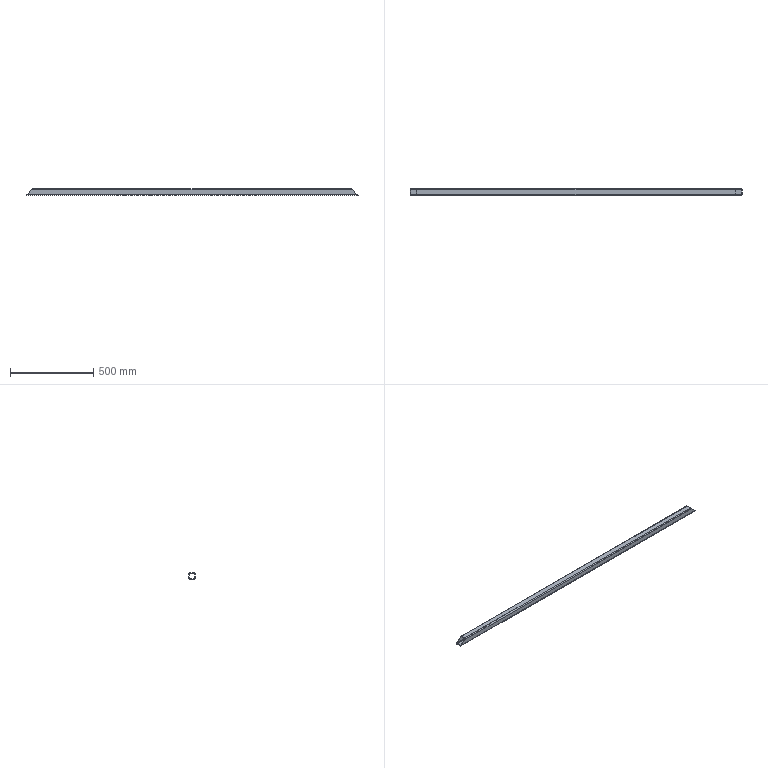Part | SolidWorks | features SavedExtBody 1 | 1 solid | 18 faces | box 2000 x 40 x 40 mm | volume 871553 mm3 | plane 10 | cylinder 8 | commonest cylinder face diameters 6.4 x4 12.8 x4
STEP:
#1=CARTESIAN_POINT('',(-1973.6,440.,-443.6));
#2=VERTEX_POINT('',#1);
#3=CARTESIAN_POINT('',(-1980.,433.6,-450.));
#4=VERTEX_POINT('',#3);
#5=CARTESIAN_POINT('',(-1973.6,440.,-443.6));
#6=CARTESIAN_POINT('',(-1977.349,440.,-447.349));
#7=CARTESIAN_POINT('',(-1980.,437.349,-450.));
#8=CARTESIAN_POINT('',(-1980.,433.6,-450.));
#9=(BOUNDED_CURVE()B_SPLINE_CURVE(3,(#5,#6,#7,#8),.UNSPECIFIED.,.F.,.F.)B_SPLINE_CURVE_WITH_KNOTS((4,4),(4.712,6.283),.UNSPECIFIED.)CURVE()GEOMETRIC_REPRESENTATION_ITEM()RATIONAL_B_SPLINE_CURVE((1.,0.8047,0.8047,1.))REPRESENTATION_ITEM(''));
#10=EDGE_CURVE('',#2,#4,#9,.T.);
#11=ORIENTED_EDGE('',*,*,#10,.F.);
#12=CARTESIAN_POINT('',(13.6,440.,-443.6));
#13=VERTEX_POINT('',#12);
#14=CARTESIAN_POINT('',(0.,440.,-443.6));
#15=DIRECTION('',(-1.,0.,0.));
#16=VECTOR('',#15,1000.);
#17=LINE('',#14,#16);
#18=EDGE_CURVE('',#13,#2,#17,.T.);
#19=ORIENTED_EDGE('',*,*,#18,.F.);
#20=CARTESIAN_POINT('',(20.,433.6,-450.));
#21=VERTEX_POINT('',#20);
#22=CARTESIAN_POINT('',(20.,433.6,-450.));
#23=CARTESIAN_POINT('',(20.,437.349,-450.));
#24=CARTESIAN_POINT('',(17.349,440.,-447.349));
#25=CARTESIAN_POINT('',(13.6,440.,-443.6));
#26=(BOUNDED_CURVE()B_SPLINE_CURVE(3,(#22,#23,#24,#25),.UNSPECIFIED.,.F.,.F.)B_SPLINE_CURVE_WITH_KNOTS((4,4),(3.142,4.712),.UNSPECIFIED.)CURVE()GEOMETRIC_REPRESENTATION_ITEM()RATIONAL_B_SPLINE_CURVE((1.,0.8047,0.8047,1.))REPRESENTATION_ITEM(''));
#27=EDGE_CURVE('',#21,#13,#26,.T.);
#28=ORIENTED_EDGE('',*,*,#27,.F.);
#29=CARTESIAN_POINT('',(0.,433.6,-450.));
#30=DIRECTION('',(-1.,0.,0.));
#31=VECTOR('',#30,1000.);
#32=LINE('',#29,#31);
#33=EDGE_CURVE('',#21,#4,#32,.T.);
#34=ORIENTED_EDGE('',*,*,#33,.T.);
#35=EDGE_LOOP('',(#11,#19,#28,#34));
#36=FACE_OUTER_BOUND('',#35,.T.);
#37=CARTESIAN_POINT('',(0.,433.6,-443.6));
#38=DIRECTION('',(-1.,0.,0.));
#39=DIRECTION('',(0.,-1.,0.));
#40=AXIS2_PLACEMENT_3D('',#37,#38,#39);
#41=CYLINDRICAL_SURFACE('',#40,6.4);
#42=ADVANCED_FACE('',(#36),#41,.T.);
#43=CARTESIAN_POINT('',(-1946.4,440.,-416.4));
#44=VERTEX_POINT('',#43);
#45=CARTESIAN_POINT('',(-986.8,440.,543.2));
#46=DIRECTION('',(-0.7071,0.,-0.7071));
#47=VECTOR('',#46,1000.);
#48=LINE('',#45,#47);
#49=EDGE_CURVE('',#44,#2,#48,.T.);
#50=ORIENTED_EDGE('',*,*,#49,.F.);
#51=CARTESIAN_POINT('',(-13.6,440.,-416.4));
#52=VERTEX_POINT('',#51);
#53=CARTESIAN_POINT('',(0.,440.,-416.4));
#54=DIRECTION('',(-1.,0.,0.));
#55=VECTOR('',#54,1000.);
#56=LINE('',#53,#55);
#57=EDGE_CURVE('',#52,#44,#56,.T.);
#58=ORIENTED_EDGE('',*,*,#57,.F.);
#59=CARTESIAN_POINT('',(6.8,440.,-436.8));
#60=DIRECTION('',(-0.7071,0.,0.7071));
#61=VECTOR('',#60,1000.);
#62=LINE('',#59,#61);
#63=EDGE_CURVE('',#13,#52,#62,.T.);
#64=ORIENTED_EDGE('',*,*,#63,.F.);
#65=ORIENTED_EDGE('',*,*,#18,.T.);
#66=EDGE_LOOP('',(#50,#58,#64,#65));
#67=FACE_OUTER_BOUND('',#66,.T.);
#68=CARTESIAN_POINT('',(0.,440.,-443.6));
#69=DIRECTION('',(0.,-1.,0.));
#70=DIRECTION('',(1.,0.,0.));
#71=AXIS2_PLACEMENT_3D('',#68,#69,#70);
#72=PLANE('',#71);
#73=ADVANCED_FACE('',(#67),#72,.F.);
#74=CARTESIAN_POINT('',(-1940.,433.6,-410.));
#75=VERTEX_POINT('',#74);
#76=CARTESIAN_POINT('',(-1940.,433.6,-410.));
#77=CARTESIAN_POINT('',(-1940.,437.349,-410.));
#78=CARTESIAN_POINT('',(-1942.651,440.,-412.651));
#79=CARTESIAN_POINT('',(-1946.4,440.,-416.4));
#80=(BOUNDED_CURVE()B_SPLINE_CURVE(3,(#76,#77,#78,#79),.UNSPECIFIED.,.F.,.F.)B_SPLINE_CURVE_WITH_KNOTS((4,4),(3.142,4.712),.UNSPECIFIED.)CURVE()GEOMETRIC_REPRESENTATION_ITEM()RATIONAL_B_SPLINE_CURVE((1.,0.8047,0.8047,1.))REPRESENTATION_ITEM(''));
#81=EDGE_CURVE('',#75,#44,#80,.T.);
#82=ORIENTED_EDGE('',*,*,#81,.F.);
#83=CARTESIAN_POINT('',(-20.,433.6,-410.));
#84=VERTEX_POINT('',#83);
#85=CARTESIAN_POINT('',(0.,433.6,-410.));
#86=DIRECTION('',(-1.,0.,0.));
#87=VECTOR('',#86,1000.);
#88=LINE('',#85,#87);
#89=EDGE_CURVE('',#84,#75,#88,.T.);
#90=ORIENTED_EDGE('',*,*,#89,.F.);
#91=CARTESIAN_POINT('',(-13.6,440.,-416.4));
#92=CARTESIAN_POINT('',(-17.349,440.,-412.651));
#93=CARTESIAN_POINT('',(-20.,437.349,-410.));
#94=CARTESIAN_POINT('',(-20.,433.6,-410.));
#95=(BOUNDED_CURVE()B_SPLINE_CURVE(3,(#91,#92,#93,#94),.UNSPECIFIED.,.F.,.F.)B_SPLINE_CURVE_WITH_KNOTS((4,4),(4.712,6.283),.UNSPECIFIED.)CURVE()GEOMETRIC_REPRESENTATION_ITEM()RATIONAL_B_SPLINE_CURVE((1.,0.8047,0.8047,1.))REPRESENTATION_ITEM(''));
#96=EDGE_CURVE('',#52,#84,#95,.T.);
#97=ORIENTED_EDGE('',*,*,#96,.F.);
#98=ORIENTED_EDGE('',*,*,#57,.T.);
#99=EDGE_LOOP('',(#82,#90,#97,#98));
#100=FACE_OUTER_BOUND('',#99,.T.);
#101=CARTESIAN_POINT('',(0.,433.6,-416.4));
#102=DIRECTION('',(-1.,0.,0.));
#103=DIRECTION('',(0.,-1.,0.));
#104=AXIS2_PLACEMENT_3D('',#101,#102,#103);
#105=CYLINDRICAL_SURFACE('',#104,6.4);
#106=ADVANCED_FACE('',(#100),#105,.T.);
#107=CARTESIAN_POINT('',(-1940.,406.4,-410.));
#108=VERTEX_POINT('',#107);
#109=CARTESIAN_POINT('',(-1940.,406.4,-410.));
#110=DIRECTION('',(0.,1.,0.));
#111=VECTOR('',#110,1000.);
#112=LINE('',#109,#111);
#113=EDGE_CURVE('',#108,#75,#112,.T.);
#114=ORIENTED_EDGE('',*,*,#113,.F.);
#115=CARTESIAN_POINT('',(-20.,406.4,-410.));
#116=VERTEX_POINT('',#115);
#117=CARTESIAN_POINT('',(0.,406.4,-410.));
#118=DIRECTION('',(-1.,0.,0.));
#119=VECTOR('',#118,1000.);
#120=LINE('',#117,#119);
#121=EDGE_CURVE('',#116,#108,#120,.T.);
#122=ORIENTED_EDGE('',*,*,#121,.F.);
#123=CARTESIAN_POINT('',(-20.,406.4,-410.));
#124=DIRECTION('',(0.,-1.,0.));
#125=VECTOR('',#124,1000.);
#126=LINE('',#123,#125);
#127=EDGE_CURVE('',#84,#116,#126,.T.);
#128=ORIENTED_EDGE('',*,*,#127,.F.);
#129=ORIENTED_EDGE('',*,*,#89,.T.);
#130=EDGE_LOOP('',(#114,#122,#128,#129));
#131=FACE_OUTER_BOUND('',#130,.T.);
#132=CARTESIAN_POINT('',(0.,406.4,-410.));
#133=DIRECTION('',(0.,0.,-1.));
#134=DIRECTION('',(0.,1.,0.));
#135=AXIS2_PLACEMENT_3D('',#132,#133,#134);
#136=PLANE('',#135);
#137=ADVANCED_FACE('',(#131),#136,.F.);
#138=CARTESIAN_POINT('',(-1946.4,400.,-416.4));
#139=VERTEX_POINT('',#138);
#140=CARTESIAN_POINT('',(-1946.4,400.,-416.4));
#141=CARTESIAN_POINT('',(-1942.651,400.,-412.651));
#142=CARTESIAN_POINT('',(-1940.,402.651,-410.));
#143=CARTESIAN_POINT('',(-1940.,406.4,-410.));
#144=(BOUNDED_CURVE()B_SPLINE_CURVE(3,(#140,#141,#142,#143),.UNSPECIFIED.,.F.,.F.)B_SPLINE_CURVE_WITH_KNOTS((4,4),(1.571,3.142),.UNSPECIFIED.)CURVE()GEOMETRIC_REPRESENTATION_ITEM()RATIONAL_B_SPLINE_CURVE((1.,0.8047,0.8047,1.))REPRESENTATION_ITEM(''));
#145=EDGE_CURVE('',#139,#108,#144,.T.);
#146=ORIENTED_EDGE('',*,*,#145,.F.);
#147=CARTESIAN_POINT('',(-13.6,400.,-416.4));
#148=VERTEX_POINT('',#147);
#149=CARTESIAN_POINT('',(0.,400.,-416.4));
#150=DIRECTION('',(-1.,0.,0.));
#151=VECTOR('',#150,1000.);
#152=LINE('',#149,#151);
#153=EDGE_CURVE('',#148,#139,#152,.T.);
#154=ORIENTED_EDGE('',*,*,#153,.F.);
#155=CARTESIAN_POINT('',(-20.,406.4,-410.));
#156=CARTESIAN_POINT('',(-20.,402.651,-410.));
#157=CARTESIAN_POINT('',(-17.349,400.,-412.651));
#158=CARTESIAN_POINT('',(-13.6,400.,-416.4));
#159=(BOUNDED_CURVE()B_SPLINE_CURVE(3,(#155,#156,#157,#158),.UNSPECIFIED.,.F.,.F.)B_SPLINE_CURVE_WITH_KNOTS((4,4),(0.,1.571),.UNSPECIFIED.)CURVE()GEOMETRIC_REPRESENTATION_ITEM()RATIONAL_B_SPLINE_CURVE((1.,0.8047,0.8047,1.))REPRESENTATION_ITEM(''));
#160=EDGE_CURVE('',#116,#148,#159,.T.);
#161=ORIENTED_EDGE('',*,*,#160,.F.);
#162=ORIENTED_EDGE('',*,*,#121,.T.);
#163=EDGE_LOOP('',(#146,#154,#161,#162));
#164=FACE_OUTER_BOUND('',#163,.T.);
#165=CARTESIAN_POINT('',(0.,406.4,-416.4));
#166=DIRECTION('',(-1.,0.,0.));
#167=DIRECTION('',(0.,-1.,0.));
#168=AXIS2_PLACEMENT_3D('',#165,#166,#167);
#169=CYLINDRICAL_SURFACE('',#168,6.4);
#170=ADVANCED_FACE('',(#164),#169,.T.);
#171=CARTESIAN_POINT('',(-1973.6,400.,-443.6));
#172=VERTEX_POINT('',#171);
#173=CARTESIAN_POINT('',(-973.2,400.,556.8));
#174=DIRECTION('',(0.7071,0.,0.7071));
#175=VECTOR('',#174,1000.);
#176=LINE('',#173,#175);
#177=EDGE_CURVE('',#172,#139,#176,.T.);
#178=ORIENTED_EDGE('',*,*,#177,.F.);
#179=CARTESIAN_POINT('',(13.6,400.,-443.6));
#180=VERTEX_POINT('',#179);
#181=CARTESIAN_POINT('',(0.,400.,-443.6));
#182=DIRECTION('',(-1.,0.,0.));
#183=VECTOR('',#182,1000.);
#184=LINE('',#181,#183);
#185=EDGE_CURVE('',#180,#172,#184,.T.);
#186=ORIENTED_EDGE('',*,*,#185,.F.);
#187=CARTESIAN_POINT('',(-6.8,400.,-423.2));
#188=DIRECTION('',(0.7071,0.,-0.7071));
#189=VECTOR('',#188,1000.);
#190=LINE('',#187,#189);
#191=EDGE_CURVE('',#148,#180,#190,.T.);
#192=ORIENTED_EDGE('',*,*,#191,.F.);
#193=ORIENTED_EDGE('',*,*,#153,.T.);
#194=EDGE_LOOP('',(#178,#186,#192,#193));
#195=FACE_OUTER_BOUND('',#194,.T.);
#196=CARTESIAN_POINT('',(0.,400.,-416.4));
#197=DIRECTION('',(0.,1.,0.));
#198=DIRECTION('',(0.,0.,1.));
#199=AXIS2_PLACEMENT_3D('',#196,#197,#198);
#200=PLANE('',#199);
#201=ADVANCED_FACE('',(#195),#200,.F.);
#202=CARTESIAN_POINT('',(-1980.,406.4,-450.));
#203=VERTEX_POINT('',#202);
#204=CARTESIAN_POINT('',(-1980.,406.4,-450.));
#205=CARTESIAN_POINT('',(-1980.,402.651,-450.));
#206=CARTESIAN_POINT('',(-1977.349,400.,-447.349));
#207=CARTESIAN_POINT('',(-1973.6,400.,-443.6));
#208=(BOUNDED_CURVE()B_SPLINE_CURVE(3,(#204,#205,#206,#207),.UNSPECIFIED.,.F.,.F.)B_SPLINE_CURVE_WITH_KNOTS((4,4),(0.,1.571),.UNSPECIFIED.)CURVE()GEOMETRIC_REPRESENTATION_ITEM()RATIONAL_B_SPLINE_CURVE((1.,0.8047,0.8047,1.))REPRESENTATION_ITEM(''));
#209=EDGE_CURVE('',#203,#172,#208,.T.);
#210=ORIENTED_EDGE('',*,*,#209,.F.);
#211=CARTESIAN_POINT('',(20.,406.4,-450.));
#212=VERTEX_POINT('',#211);
#213=CARTESIAN_POINT('',(0.,406.4,-450.));
#214=DIRECTION('',(-1.,0.,0.));
#215=VECTOR('',#214,1000.);
#216=LINE('',#213,#215);
#217=EDGE_CURVE('',#212,#203,#216,.T.);
#218=ORIENTED_EDGE('',*,*,#217,.F.);
#219=CARTESIAN_POINT('',(13.6,400.,-443.6));
#220=CARTESIAN_POINT('',(17.349,400.,-447.349));
#221=CARTESIAN_POINT('',(20.,402.651,-450.));
#222=CARTESIAN_POINT('',(20.,406.4,-450.));
#223=(BOUNDED_CURVE()B_SPLINE_CURVE(3,(#219,#220,#221,#222),.UNSPECIFIED.,.F.,.F.)B_SPLINE_CURVE_WITH_KNOTS((4,4),(1.571,3.142),.UNSPECIFIED.)CURVE()GEOMETRIC_REPRESENTATION_ITEM()RATIONAL_B_SPLINE_CURVE((1.,0.8047,0.8047,1.))REPRESENTATION_ITEM(''));
#224=EDGE_CURVE('',#180,#212,#223,.T.);
#225=ORIENTED_EDGE('',*,*,#224,.F.);
#226=ORIENTED_EDGE('',*,*,#185,.T.);
#227=EDGE_LOOP('',(#210,#218,#225,#226));
#228=FACE_OUTER_BOUND('',#227,.T.);
#229=CARTESIAN_POINT('',(0.,406.4,-443.6));
#230=DIRECTION('',(-1.,0.,0.));
#231=DIRECTION('',(0.,-1.,0.));
#232=AXIS2_PLACEMENT_3D('',#229,#230,#231);
#233=CYLINDRICAL_SURFACE('',#232,6.4);
#234=ADVANCED_FACE('',(#228),#233,.T.);
#235=CARTESIAN_POINT('',(-16.8,433.6,-413.2));
#236=VERTEX_POINT('',#235);
#237=CARTESIAN_POINT('',(-1943.2,433.6,-413.2));
#238=VERTEX_POINT('',#237);
#239=CARTESIAN_POINT('',(0.,433.6,-413.2));
#240=DIRECTION('',(-1.,0.,0.));
#241=VECTOR('',#240,1000.);
#242=LINE('',#239,#241);
#243=EDGE_CURVE('',#236,#238,#242,.T.);
#244=ORIENTED_EDGE('',*,*,#243,.T.);
#245=CARTESIAN_POINT('',(-1946.4,436.8,-416.4));
#246=VERTEX_POINT('',#245);
#247=CARTESIAN_POINT('',(-1943.2,433.6,-413.2));
#248=CARTESIAN_POINT('',(-1943.2,435.475,-413.2));
#249=CARTESIAN_POINT('',(-1944.525,436.8,-414.525));
#250=CARTESIAN_POINT('',(-1946.4,436.8,-416.4));
#251=(BOUNDED_CURVE()B_SPLINE_CURVE(3,(#247,#248,#249,#250),.UNSPECIFIED.,.F.,.F.)B_SPLINE_CURVE_WITH_KNOTS((4,4),(3.142,4.712),.UNSPECIFIED.)CURVE()GEOMETRIC_REPRESENTATION_ITEM()RATIONAL_B_SPLINE_CURVE((1.,0.8047,0.8047,1.))REPRESENTATION_ITEM(''));
#252=EDGE_CURVE('',#238,#246,#251,.T.);
#253=ORIENTED_EDGE('',*,*,#252,.T.);
#254=CARTESIAN_POINT('',(-13.6,436.8,-416.4));
#255=VERTEX_POINT('',#254);
#256=CARTESIAN_POINT('',(0.,436.8,-416.4));
#257=DIRECTION('',(-1.,0.,0.));
#258=VECTOR('',#257,1000.);
#259=LINE('',#256,#258);
#260=EDGE_CURVE('',#255,#246,#259,.T.);
#261=ORIENTED_EDGE('',*,*,#260,.F.);
#262=CARTESIAN_POINT('',(-13.6,436.8,-416.4));
#263=CARTESIAN_POINT('',(-15.475,436.8,-414.525));
#264=CARTESIAN_POINT('',(-16.8,435.475,-413.2));
#265=CARTESIAN_POINT('',(-16.8,433.6,-413.2));
#266=(BOUNDED_CURVE()B_SPLINE_CURVE(3,(#262,#263,#264,#265),.UNSPECIFIED.,.F.,.F.)B_SPLINE_CURVE_WITH_KNOTS((4,4),(4.712,6.283),.UNSPECIFIED.)CURVE()GEOMETRIC_REPRESENTATION_ITEM()RATIONAL_B_SPLINE_CURVE((1.,0.8047,0.8047,1.))REPRESENTATION_ITEM(''));
#267=EDGE_CURVE('',#255,#236,#266,.T.);
#268=ORIENTED_EDGE('',*,*,#267,.T.);
#269=EDGE_LOOP('',(#244,#253,#261,#268));
#270=FACE_OUTER_BOUND('',#269,.T.);
#271=CARTESIAN_POINT('',(0.,433.6,-416.4));
#272=DIRECTION('',(-1.,0.,0.));
#273=DIRECTION('',(0.,-1.,0.));
#274=AXIS2_PLACEMENT_3D('',#271,#272,#273);
#275=CYLINDRICAL_SURFACE('',#274,3.2);
#276=ADVANCED_FACE('',(#270),#275,.F.);
#277=ORIENTED_EDGE('',*,*,#260,.T.);
#278=CARTESIAN_POINT('',(-1973.6,436.8,-443.6));
#279=VERTEX_POINT('',#278);
#280=CARTESIAN_POINT('',(-986.8,436.8,543.2));
#281=DIRECTION('',(-0.7071,0.,-0.7071));
#282=VECTOR('',#281,1000.);
#283=LINE('',#280,#282);
#284=EDGE_CURVE('',#246,#279,#283,.T.);
#285=ORIENTED_EDGE('',*,*,#284,.T.);
#286=CARTESIAN_POINT('',(13.6,436.8,-443.6));
#287=VERTEX_POINT('',#286);
#288=CARTESIAN_POINT('',(0.,436.8,-443.6));
#289=DIRECTION('',(-1.,0.,0.));
#290=VECTOR('',#289,1000.);
#291=LINE('',#288,#290);
#292=EDGE_CURVE('',#287,#279,#291,.T.);
#293=ORIENTED_EDGE('',*,*,#292,.F.);
#294=CARTESIAN_POINT('',(6.8,436.8,-436.8));
#295=DIRECTION('',(-0.7071,0.,0.7071));
#296=VECTOR('',#295,1000.);
#297=LINE('',#294,#296);
#298=EDGE_CURVE('',#287,#255,#297,.T.);
#299=ORIENTED_EDGE('',*,*,#298,.T.);
#300=EDGE_LOOP('',(#277,#285,#293,#299));
#301=FACE_OUTER_BOUND('',#300,.T.);
#302=CARTESIAN_POINT('',(0.,436.8,-443.6));
#303=DIRECTION('',(0.,-1.,0.));
#304=DIRECTION('',(1.,0.,0.));
#305=AXIS2_PLACEMENT_3D('',#302,#303,#304);
#306=PLANE('',#305);
#307=ADVANCED_FACE('',(#301),#306,.T.);
#308=ORIENTED_EDGE('',*,*,#292,.T.);
#309=CARTESIAN_POINT('',(-1976.8,433.6,-446.8));
#310=VERTEX_POINT('',#309);
#311=CARTESIAN_POINT('',(-1973.6,436.8,-443.6));
#312=CARTESIAN_POINT('',(-1975.475,436.8,-445.475));
#313=CARTESIAN_POINT('',(-1976.8,435.475,-446.8));
#314=CARTESIAN_POINT('',(-1976.8,433.6,-446.8));
#315=(BOUNDED_CURVE()B_SPLINE_CURVE(3,(#311,#312,#313,#314),.UNSPECIFIED.,.F.,.F.)B_SPLINE_CURVE_WITH_KNOTS((4,4),(4.712,6.283),.UNSPECIFIED.)CURVE()GEOMETRIC_REPRESENTATION_ITEM()RATIONAL_B_SPLINE_CURVE((1.,0.8047,0.8047,1.))REPRESENTATION_ITEM(''));
#316=EDGE_CURVE('',#279,#310,#315,.T.);
#317=ORIENTED_EDGE('',*,*,#316,.T.);
#318=CARTESIAN_POINT('',(16.8,433.6,-446.8));
#319=VERTEX_POINT('',#318);
#320=CARTESIAN_POINT('',(0.,433.6,-446.8));
#321=DIRECTION('',(-1.,0.,0.));
#322=VECTOR('',#321,1000.);
#323=LINE('',#320,#322);
#324=EDGE_CURVE('',#319,#310,#323,.T.);
#325=ORIENTED_EDGE('',*,*,#324,.F.);
#326=CARTESIAN_POINT('',(16.8,433.6,-446.8));
#327=CARTESIAN_POINT('',(16.8,435.475,-446.8));
#328=CARTESIAN_POINT('',(15.475,436.8,-445.475));
#329=CARTESIAN_POINT('',(13.6,436.8,-443.6));
#330=(BOUNDED_CURVE()B_SPLINE_CURVE(3,(#326,#327,#328,#329),.UNSPECIFIED.,.F.,.T.)B_SPLINE_CURVE_WITH_KNOTS((4,4),(3.142,4.712),.UNSPECIFIED.)CURVE()GEOMETRIC_REPRESENTATION_ITEM()RATIONAL_B_SPLINE_CURVE((1.,0.8047,0.8047,1.))REPRESENTATION_ITEM(''));
#331=EDGE_CURVE('',#319,#287,#330,.T.);
#332=ORIENTED_EDGE('',*,*,#331,.T.);
#333=EDGE_LOOP('',(#308,#317,#325,#332));
#334=FACE_OUTER_BOUND('',#333,.T.);
#335=CARTESIAN_POINT('',(0.,433.6,-443.6));
#336=DIRECTION('',(-1.,0.,0.));
#337=DIRECTION('',(0.,-1.,0.));
#338=AXIS2_PLACEMENT_3D('',#335,#336,#337);
#339=CYLINDRICAL_SURFACE('',#338,3.2);
#340=ADVANCED_FACE('',(#334),#339,.F.);
#341=ORIENTED_EDGE('',*,*,#324,.T.);
#342=CARTESIAN_POINT('',(-1976.8,406.4,-446.8));
#343=VERTEX_POINT('',#342);
#344=CARTESIAN_POINT('',(-1976.8,433.6,-446.8));
#345=DIRECTION('',(0.,-1.,0.));
#346=VECTOR('',#345,1000.);
#347=LINE('',#344,#346);
#348=EDGE_CURVE('',#310,#343,#347,.T.);
#349=ORIENTED_EDGE('',*,*,#348,.T.);
#350=CARTESIAN_POINT('',(16.8,406.4,-446.8));
#351=VERTEX_POINT('',#350);
#352=CARTESIAN_POINT('',(0.,406.4,-446.8));
#353=DIRECTION('',(-1.,0.,0.));
#354=VECTOR('',#353,1000.);
#355=LINE('',#352,#354);
#356=EDGE_CURVE('',#351,#343,#355,.T.);
#357=ORIENTED_EDGE('',*,*,#356,.F.);
#358=CARTESIAN_POINT('',(16.8,433.6,-446.8));
#359=DIRECTION('',(0.,1.,0.));
#360=VECTOR('',#359,1000.);
#361=LINE('',#358,#360);
#362=EDGE_CURVE('',#351,#319,#361,.T.);
#363=ORIENTED_EDGE('',*,*,#362,.T.);
#364=EDGE_LOOP('',(#341,#349,#357,#363));
#365=FACE_OUTER_BOUND('',#364,.T.);
#366=CARTESIAN_POINT('',(0.,433.6,-446.8));
#367=DIRECTION('',(0.,0.,1.));
#368=DIRECTION('',(0.,-1.,0.));
#369=AXIS2_PLACEMENT_3D('',#366,#367,#368);
#370=PLANE('',#369);
#371=ADVANCED_FACE('',(#365),#370,.T.);
#372=ORIENTED_EDGE('',*,*,#356,.T.);
#373=CARTESIAN_POINT('',(-1973.6,403.2,-443.6));
#374=VERTEX_POINT('',#373);
#375=CARTESIAN_POINT('',(-1976.8,406.4,-446.8));
#376=CARTESIAN_POINT('',(-1976.8,404.525,-446.8));
#377=CARTESIAN_POINT('',(-1975.475,403.2,-445.475));
#378=CARTESIAN_POINT('',(-1973.6,403.2,-443.6));
#379=(BOUNDED_CURVE()B_SPLINE_CURVE(3,(#375,#376,#377,#378),.UNSPECIFIED.,.F.,.F.)B_SPLINE_CURVE_WITH_KNOTS((4,4),(0.,1.571),.UNSPECIFIED.)CURVE()GEOMETRIC_REPRESENTATION_ITEM()RATIONAL_B_SPLINE_CURVE((1.,0.8047,0.8047,1.))REPRESENTATION_ITEM(''));
#380=EDGE_CURVE('',#343,#374,#379,.T.);
#381=ORIENTED_EDGE('',*,*,#380,.T.);
#382=CARTESIAN_POINT('',(13.6,403.2,-443.6));
#383=VERTEX_POINT('',#382);
#384=CARTESIAN_POINT('',(0.,403.2,-443.6));
#385=DIRECTION('',(-1.,0.,0.));
#386=VECTOR('',#385,1000.);
#387=LINE('',#384,#386);
#388=EDGE_CURVE('',#383,#374,#387,.T.);
#389=ORIENTED_EDGE('',*,*,#388,.F.);
#390=CARTESIAN_POINT('',(13.6,403.2,-443.6));
#391=CARTESIAN_POINT('',(15.475,403.2,-445.475));
#392=CARTESIAN_POINT('',(16.8,404.525,-446.8));
#393=CARTESIAN_POINT('',(16.8,406.4,-446.8));
#394=(BOUNDED_CURVE()B_SPLINE_CURVE(3,(#390,#391,#392,#393),.UNSPECIFIED.,.F.,.F.)B_SPLINE_CURVE_WITH_KNOTS((4,4),(1.571,3.142),.UNSPECIFIED.)CURVE()GEOMETRIC_REPRESENTATION_ITEM()RATIONAL_B_SPLINE_CURVE((1.,0.8047,0.8047,1.))REPRESENTATION_ITEM(''));
#395=EDGE_CURVE('',#383,#351,#394,.T.);
#396=ORIENTED_EDGE('',*,*,#395,.T.);
#397=EDGE_LOOP('',(#372,#381,#389,#396));
#398=FACE_OUTER_BOUND('',#397,.T.);
#399=CARTESIAN_POINT('',(0.,406.4,-443.6));
#400=DIRECTION('',(-1.,0.,0.));
#401=DIRECTION('',(0.,-1.,0.));
#402=AXIS2_PLACEMENT_3D('',#399,#400,#401);
#403=CYLINDRICAL_SURFACE('',#402,3.2);
#404=ADVANCED_FACE('',(#398),#403,.F.);
#405=ORIENTED_EDGE('',*,*,#388,.T.);
#406=CARTESIAN_POINT('',(-1946.4,403.2,-416.4));
#407=VERTEX_POINT('',#406);
#408=CARTESIAN_POINT('',(-973.2,403.2,556.8));
#409=DIRECTION('',(0.7071,0.,0.7071));
#410=VECTOR('',#409,1000.);
#411=LINE('',#408,#410);
#412=EDGE_CURVE('',#374,#407,#411,.T.);
#413=ORIENTED_EDGE('',*,*,#412,.T.);
#414=CARTESIAN_POINT('',(-13.6,403.2,-416.4));
#415=VERTEX_POINT('',#414);
#416=CARTESIAN_POINT('',(0.,403.2,-416.4));
#417=DIRECTION('',(-1.,0.,0.));
#418=VECTOR('',#417,1000.);
#419=LINE('',#416,#418);
#420=EDGE_CURVE('',#415,#407,#419,.T.);
#421=ORIENTED_EDGE('',*,*,#420,.F.);
#422=CARTESIAN_POINT('',(-6.8,403.2,-423.2));
#423=DIRECTION('',(0.7071,0.,-0.7071));
#424=VECTOR('',#423,1000.);
#425=LINE('',#422,#424);
#426=EDGE_CURVE('',#415,#383,#425,.T.);
#427=ORIENTED_EDGE('',*,*,#426,.T.);
#428=EDGE_LOOP('',(#405,#413,#421,#427));
#429=FACE_OUTER_BOUND('',#428,.T.);
#430=CARTESIAN_POINT('',(0.,403.2,-416.4));
#431=DIRECTION('',(0.,1.,0.));
#432=DIRECTION('',(0.,0.,1.));
#433=AXIS2_PLACEMENT_3D('',#430,#431,#432);
#434=PLANE('',#433);
#435=ADVANCED_FACE('',(#429),#434,.T.);
#436=ORIENTED_EDGE('',*,*,#420,.T.);
#437=CARTESIAN_POINT('',(-1943.2,406.4,-413.2));
#438=VERTEX_POINT('',#437);
#439=CARTESIAN_POINT('',(-1946.4,403.2,-416.4));
#440=CARTESIAN_POINT('',(-1944.525,403.2,-414.525));
#441=CARTESIAN_POINT('',(-1943.2,404.525,-413.2));
#442=CARTESIAN_POINT('',(-1943.2,406.4,-413.2));
#443=(BOUNDED_CURVE()B_SPLINE_CURVE(3,(#439,#440,#441,#442),.UNSPECIFIED.,.F.,.F.)B_SPLINE_CURVE_WITH_KNOTS((4,4),(1.571,3.142),.UNSPECIFIED.)CURVE()GEOMETRIC_REPRESENTATION_ITEM()RATIONAL_B_SPLINE_CURVE((1.,0.8047,0.8047,1.))REPRESENTATION_ITEM(''));
#444=EDGE_CURVE('',#407,#438,#443,.T.);
#445=ORIENTED_EDGE('',*,*,#444,.T.);
#446=CARTESIAN_POINT('',(-16.8,406.4,-413.2));
#447=VERTEX_POINT('',#446);
#448=CARTESIAN_POINT('',(0.,406.4,-413.2));
#449=DIRECTION('',(-1.,0.,0.));
#450=VECTOR('',#449,1000.);
#451=LINE('',#448,#450);
#452=EDGE_CURVE('',#447,#438,#451,.T.);
#453=ORIENTED_EDGE('',*,*,#452,.F.);
#454=CARTESIAN_POINT('',(-16.8,406.4,-413.2));
#455=CARTESIAN_POINT('',(-16.8,404.525,-413.2));
#456=CARTESIAN_POINT('',(-15.475,403.2,-414.525));
#457=CARTESIAN_POINT('',(-13.6,403.2,-416.4));
#458=(BOUNDED_CURVE()B_SPLINE_CURVE(3,(#454,#455,#456,#457),.UNSPECIFIED.,.F.,.F.)B_SPLINE_CURVE_WITH_KNOTS((4,4),(0.,1.571),.UNSPECIFIED.)CURVE()GEOMETRIC_REPRESENTATION_ITEM()RATIONAL_B_SPLINE_CURVE((1.,0.8047,0.8047,1.))REPRESENTATION_ITEM(''));
#459=EDGE_CURVE('',#447,#415,#458,.T.);
#460=ORIENTED_EDGE('',*,*,#459,.T.);
#461=EDGE_LOOP('',(#436,#445,#453,#460));
#462=FACE_OUTER_BOUND('',#461,.T.);
#463=CARTESIAN_POINT('',(0.,406.4,-416.4));
#464=DIRECTION('',(-1.,0.,0.));
#465=DIRECTION('',(0.,-1.,0.));
#466=AXIS2_PLACEMENT_3D('',#463,#464,#465);
#467=CYLINDRICAL_SURFACE('',#466,3.2);
#468=ADVANCED_FACE('',(#462),#467,.F.);
#469=ORIENTED_EDGE('',*,*,#452,.T.);
#470=CARTESIAN_POINT('',(-1943.2,406.4,-413.2));
#471=DIRECTION('',(0.,1.,0.));
#472=VECTOR('',#471,1000.);
#473=LINE('',#470,#472);
#474=EDGE_CURVE('',#438,#238,#473,.T.);
#475=ORIENTED_EDGE('',*,*,#474,.T.);
#476=ORIENTED_EDGE('',*,*,#243,.F.);
#477=CARTESIAN_POINT('',(-16.8,406.4,-413.2));
#478=DIRECTION('',(0.,-1.,0.));
#479=VECTOR('',#478,1000.);
#480=LINE('',#477,#479);
#481=EDGE_CURVE('',#236,#447,#480,.T.);
#482=ORIENTED_EDGE('',*,*,#481,.T.);
#483=EDGE_LOOP('',(#469,#475,#476,#482));
#484=FACE_OUTER_BOUND('',#483,.T.);
#485=CARTESIAN_POINT('',(0.,406.4,-413.2));
#486=DIRECTION('',(0.,0.,-1.));
#487=DIRECTION('',(0.,1.,0.));
#488=AXIS2_PLACEMENT_3D('',#485,#486,#487);
#489=PLANE('',#488);
#490=ADVANCED_FACE('',(#484),#489,.T.);
#491=CARTESIAN_POINT('',(-1980.,433.6,-450.));
#492=DIRECTION('',(0.,-1.,0.));
#493=VECTOR('',#492,1000.);
#494=LINE('',#491,#493);
#495=EDGE_CURVE('',#4,#203,#494,.T.);
#496=ORIENTED_EDGE('',*,*,#495,.F.);
#497=ORIENTED_EDGE('',*,*,#33,.F.);
#498=CARTESIAN_POINT('',(20.,433.6,-450.));
#499=DIRECTION('',(0.,1.,0.));
#500=VECTOR('',#499,1000.);
#501=LINE('',#498,#500);
#502=EDGE_CURVE('',#212,#21,#501,.T.);
#503=ORIENTED_EDGE('',*,*,#502,.F.);
#504=ORIENTED_EDGE('',*,*,#217,.T.);
#505=EDGE_LOOP('',(#496,#497,#503,#504));
#506=FACE_OUTER_BOUND('',#505,.T.);
#507=CARTESIAN_POINT('',(0.,433.6,-450.));
#508=DIRECTION('',(0.,0.,1.));
#509=DIRECTION('',(0.,-1.,0.));
#510=AXIS2_PLACEMENT_3D('',#507,#508,#509);
#511=PLANE('',#510);
#512=ADVANCED_FACE('',(#506),#511,.F.);
#513=ORIENTED_EDGE('',*,*,#267,.F.);
#514=ORIENTED_EDGE('',*,*,#298,.F.);
#515=ORIENTED_EDGE('',*,*,#331,.F.);
#516=ORIENTED_EDGE('',*,*,#362,.F.);
#517=ORIENTED_EDGE('',*,*,#395,.F.);
#518=ORIENTED_EDGE('',*,*,#426,.F.);
#519=ORIENTED_EDGE('',*,*,#459,.F.);
#520=ORIENTED_EDGE('',*,*,#481,.F.);
#521=EDGE_LOOP('',(#513,#514,#515,#516,#517,#518,#519,#520));
#522=FACE_BOUND('',#521,.T.);
#523=ORIENTED_EDGE('',*,*,#502,.T.);
#524=ORIENTED_EDGE('',*,*,#27,.T.);
#525=ORIENTED_EDGE('',*,*,#63,.T.);
#526=ORIENTED_EDGE('',*,*,#96,.T.);
#527=ORIENTED_EDGE('',*,*,#127,.T.);
#528=ORIENTED_EDGE('',*,*,#160,.T.);
#529=ORIENTED_EDGE('',*,*,#191,.T.);
#530=ORIENTED_EDGE('',*,*,#224,.T.);
#531=EDGE_LOOP('',(#523,#524,#525,#526,#527,#528,#529,#530));
#532=FACE_OUTER_BOUND('',#531,.T.);
#533=CARTESIAN_POINT('',(0.,420.,-430.));
#534=DIRECTION('',(0.7071,0.,0.7071));
#535=DIRECTION('',(0.7071,0.,-0.7071));
#536=AXIS2_PLACEMENT_3D('',#533,#534,#535);
#537=PLANE('',#536);
#538=ADVANCED_FACE('',(#522,#532),#537,.T.);
#539=ORIENTED_EDGE('',*,*,#252,.F.);
#540=ORIENTED_EDGE('',*,*,#474,.F.);
#541=ORIENTED_EDGE('',*,*,#444,.F.);
#542=ORIENTED_EDGE('',*,*,#412,.F.);
#543=ORIENTED_EDGE('',*,*,#380,.F.);
#544=ORIENTED_EDGE('',*,*,#348,.F.);
#545=ORIENTED_EDGE('',*,*,#316,.F.);
#546=ORIENTED_EDGE('',*,*,#284,.F.);
#547=EDGE_LOOP('',(#539,#540,#541,#542,#543,#544,#545,#546));
#548=FACE_BOUND('',#547,.T.);
#549=ORIENTED_EDGE('',*,*,#49,.T.);
#550=ORIENTED_EDGE('',*,*,#10,.T.);
#551=ORIENTED_EDGE('',*,*,#495,.T.);
#552=ORIENTED_EDGE('',*,*,#209,.T.);
#553=ORIENTED_EDGE('',*,*,#177,.T.);
#554=ORIENTED_EDGE('',*,*,#145,.T.);
#555=ORIENTED_EDGE('',*,*,#113,.T.);
#556=ORIENTED_EDGE('',*,*,#81,.T.);
#557=EDGE_LOOP('',(#549,#550,#551,#552,#553,#554,#555,#556));
#558=FACE_OUTER_BOUND('',#557,.T.);
#559=CARTESIAN_POINT('',(-1960.,420.,-430.));
#560=DIRECTION('',(-0.7071,0.,0.7071));
#561=DIRECTION('',(0.7071,0.,0.7071));
#562=AXIS2_PLACEMENT_3D('',#559,#560,#561);
#563=PLANE('',#562);
#564=ADVANCED_FACE('',(#548,#558),#563,.T.);
#565=CLOSED_SHELL('',(#42,#73,#106,#137,#170,#201,#234,#276,#307,#340,#371,#404,#435,#468,#490,#512,#538,#564));
#566=MANIFOLD_SOLID_BREP('',#565);
#567=CARTESIAN_POINT('',(0.,0.,0.));
#568=DIRECTION('',(0.,0.,1.));
#569=DIRECTION('',(1.,0.,0.));
#570=AXIS2_PLACEMENT_3D('',#567,#568,#569);
#571=(LENGTH_UNIT()NAMED_UNIT(*)SI_UNIT(.MILLI.,.METRE.));
#572=UNCERTAINTY_MEASURE_WITH_UNIT(LENGTH_MEASURE(0.00001),#571,'','');
#573=(NAMED_UNIT(*)PLANE_ANGLE_UNIT()SI_UNIT($,.RADIAN.));
#574=(NAMED_UNIT(*)SI_UNIT($,.STERADIAN.)SOLID_ANGLE_UNIT());
#575=(GEOMETRIC_REPRESENTATION_CONTEXT(3)GLOBAL_UNCERTAINTY_ASSIGNED_CONTEXT((#572))GLOBAL_UNIT_ASSIGNED_CONTEXT((#571,#573,#574))REPRESENTATION_CONTEXT('',''));
#576=ADVANCED_BREP_SHAPE_REPRESENTATION('',(#566,#570),#575);